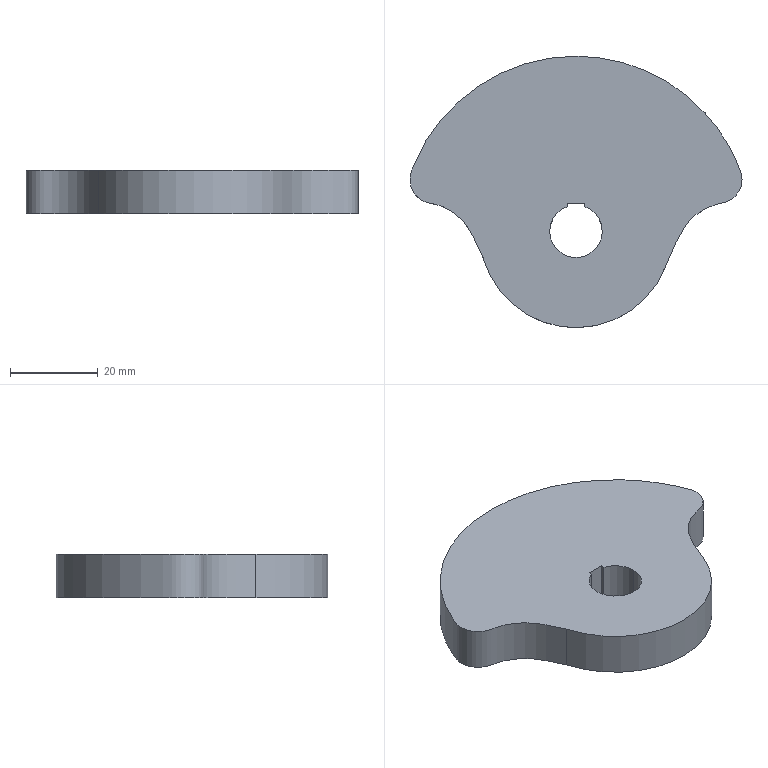Part | SolidWorks | features Extrusion 1, ICE 1 | 1 solid | 10 faces | box 75.848 x 62.021 x 10 mm | volume 29978 mm3 | plane 5 | cylinder 3 | spline 2 | commonest cylinder face diameters 12 x3
STEP:
#1=CARTESIAN_POINT('',(-6.,0.,0.));
#2=VERTEX_POINT('',#1);
#3=CARTESIAN_POINT('',(6.,0.,0.));
#4=VERTEX_POINT('',#3);
#5=CARTESIAN_POINT('',(0.,0.,0.));
#6=DIRECTION('',(0.,0.,1.));
#7=DIRECTION('',(-1.,0.,0.));
#8=AXIS2_PLACEMENT_3D('',#5,#6,#7);
#9=CIRCLE('',#8,6.);
#10=EDGE_CURVE('',#2,#4,#9,.T.);
#11=ORIENTED_EDGE('',*,*,#10,.F.);
#12=CARTESIAN_POINT('',(-6.,0.,10.));
#13=VERTEX_POINT('',#12);
#14=CARTESIAN_POINT('',(-6.,0.,-113.18));
#15=DIRECTION('',(0.,0.,1.));
#16=VECTOR('',#15,1000.);
#17=LINE('',#14,#16);
#18=EDGE_CURVE('',#2,#13,#17,.T.);
#19=ORIENTED_EDGE('',*,*,#18,.T.);
#20=CARTESIAN_POINT('',(6.,0.,10.));
#21=VERTEX_POINT('',#20);
#22=CARTESIAN_POINT('',(0.,0.,10.));
#23=DIRECTION('',(0.,0.,1.));
#24=DIRECTION('',(1.,0.,0.));
#25=AXIS2_PLACEMENT_3D('',#22,#23,#24);
#26=CIRCLE('',#25,6.);
#27=EDGE_CURVE('',#13,#21,#26,.T.);
#28=ORIENTED_EDGE('',*,*,#27,.T.);
#29=CARTESIAN_POINT('',(6.,0.,-113.18));
#30=DIRECTION('',(0.,0.,1.));
#31=VECTOR('',#30,1000.);
#32=LINE('',#29,#31);
#33=EDGE_CURVE('',#4,#21,#32,.T.);
#34=ORIENTED_EDGE('',*,*,#33,.F.);
#35=EDGE_LOOP('',(#11,#19,#28,#34));
#36=FACE_OUTER_BOUND('',#35,.T.);
#37=CARTESIAN_POINT('',(0.,0.,-113.18));
#38=DIRECTION('',(0.,0.,1.));
#39=DIRECTION('',(1.,0.,0.));
#40=AXIS2_PLACEMENT_3D('',#37,#38,#39);
#41=CYLINDRICAL_SURFACE('',#40,6.);
#42=ADVANCED_FACE('',(#36),#41,.F.);
#43=CARTESIAN_POINT('',(2.,5.657,0.));
#44=VERTEX_POINT('',#43);
#45=CARTESIAN_POINT('',(0.,0.,0.));
#46=DIRECTION('',(0.,0.,1.));
#47=DIRECTION('',(-1.,0.,0.));
#48=AXIS2_PLACEMENT_3D('',#45,#46,#47);
#49=CIRCLE('',#48,6.);
#50=EDGE_CURVE('',#4,#44,#49,.T.);
#51=ORIENTED_EDGE('',*,*,#50,.F.);
#52=ORIENTED_EDGE('',*,*,#33,.T.);
#53=CARTESIAN_POINT('',(2.,5.657,10.));
#54=VERTEX_POINT('',#53);
#55=CARTESIAN_POINT('',(0.,0.,10.));
#56=DIRECTION('',(0.,0.,1.));
#57=DIRECTION('',(1.,0.,0.));
#58=AXIS2_PLACEMENT_3D('',#55,#56,#57);
#59=CIRCLE('',#58,6.);
#60=EDGE_CURVE('',#21,#54,#59,.T.);
#61=ORIENTED_EDGE('',*,*,#60,.T.);
#62=CARTESIAN_POINT('',(2.,5.657,-113.18));
#63=DIRECTION('',(0.,0.,1.));
#64=VECTOR('',#63,1000.);
#65=LINE('',#62,#64);
#66=EDGE_CURVE('',#44,#54,#65,.T.);
#67=ORIENTED_EDGE('',*,*,#66,.F.);
#68=EDGE_LOOP('',(#51,#52,#61,#67));
#69=FACE_OUTER_BOUND('',#68,.T.);
#70=CARTESIAN_POINT('',(0.,0.,-113.18));
#71=DIRECTION('',(0.,0.,1.));
#72=DIRECTION('',(1.,0.,0.));
#73=AXIS2_PLACEMENT_3D('',#70,#71,#72);
#74=CYLINDRICAL_SURFACE('',#73,6.);
#75=ADVANCED_FACE('',(#69),#74,.F.);
#76=CARTESIAN_POINT('',(-21.423,-5.617,0.));
#77=VERTEX_POINT('',#76);
#78=CARTESIAN_POINT('',(29.487,27.043,0.));
#79=VERTEX_POINT('',#78);
#80=CARTESIAN_POINT('',(-21.423,-5.617,0.));
#81=CARTESIAN_POINT('',(-21.246,-6.047,0.));
#82=CARTESIAN_POINT('',(-20.905,-6.913,0.));
#83=CARTESIAN_POINT('',(-20.431,-8.228,0.));
#84=CARTESIAN_POINT('',(-20.056,-9.081,0.));
#85=CARTESIAN_POINT('',(-19.855,-9.501,0.));
#86=CARTESIAN_POINT('',(-10.656,-28.723,0.));
#87=CARTESIAN_POINT('',(10.654,-28.724,0.));
#88=CARTESIAN_POINT('',(19.854,-9.503,0.));
#89=CARTESIAN_POINT('',(20.055,-9.083,0.));
#90=CARTESIAN_POINT('',(20.43,-8.23,0.));
#91=CARTESIAN_POINT('',(20.904,-6.915,0.));
#92=CARTESIAN_POINT('',(21.246,-6.048,0.));
#93=CARTESIAN_POINT('',(21.422,-5.618,0.));
#94=CARTESIAN_POINT('',(21.978,-4.264,0.));
#95=CARTESIAN_POINT('',(22.591,-2.935,0.));
#96=CARTESIAN_POINT('',(23.261,-1.633,0.));
#97=CARTESIAN_POINT('',(23.355,-1.451,0.));
#98=CARTESIAN_POINT('',(23.545,-1.086,0.));
#99=CARTESIAN_POINT('',(23.838,-0.5418,0.));
#100=CARTESIAN_POINT('',(24.037,-0.1817,0.));
#101=CARTESIAN_POINT('',(24.138,-0.002216,0.));
#102=CARTESIAN_POINT('',(24.278,0.2481,0.));
#103=CARTESIAN_POINT('',(24.564,0.7463,0.));
#104=CARTESIAN_POINT('',(25.073,1.448,0.));
#105=CARTESIAN_POINT('',(25.433,1.896,0.));
#106=CARTESIAN_POINT('',(25.621,2.113,0.));
#107=CARTESIAN_POINT('',(27.42,4.203,0.));
#108=CARTESIAN_POINT('',(29.774,5.638,0.));
#109=CARTESIAN_POINT('',(32.456,6.278,0.));
#110=CARTESIAN_POINT('',(32.638,6.322,0.));
#111=CARTESIAN_POINT('',(33.005,6.401,0.));
#112=CARTESIAN_POINT('',(33.563,6.488,0.));
#113=CARTESIAN_POINT('',(33.927,6.581,0.));
#114=CARTESIAN_POINT('',(34.106,6.637,0.));
#115=CARTESIAN_POINT('',(36.786,7.474,0.));
#116=CARTESIAN_POINT('',(38.278,9.853,0.));
#117=CARTESIAN_POINT('',(37.865,12.631,0.));
#118=CARTESIAN_POINT('',(37.847,12.748,0.));
#119=CARTESIAN_POINT('',(37.805,12.98,0.));
#120=CARTESIAN_POINT('',(37.726,13.329,0.));
#121=CARTESIAN_POINT('',(37.646,13.552,0.));
#122=CARTESIAN_POINT('',(37.606,13.663,0.));
#123=CARTESIAN_POINT('',(37.565,13.775,0.));
#124=CARTESIAN_POINT('',(37.482,13.999,0.));
#125=CARTESIAN_POINT('',(37.356,14.333,0.));
#126=CARTESIAN_POINT('',(37.269,14.556,0.));
#127=CARTESIAN_POINT('',(37.226,14.667,0.));
#128=CARTESIAN_POINT('',(35.485,19.085,0.));
#129=CARTESIAN_POINT('',(32.926,23.294,0.));
#130=CARTESIAN_POINT('',(29.487,27.043,0.));
#131=(BOUNDED_CURVE()B_SPLINE_CURVE(3,(#80,#81,#82,#83,#84,#85,#86,#87,#88,#89,#90,#91,#92,#93,#94,#95,#96,#97,#98,#99,#100,#101,#102,#103,#104,#105,#106,#107,#108,#109,#110,#111,#112,#113,#114,#115,#116,#117,#118,#119,#120,#121,#122,#123,#124,#125,#126,#127,#128,#129,#130),.UNSPECIFIED.,.F.,.F.)B_SPLINE_CURVE_WITH_KNOTS((4,1,1,3,3,1,1,3,3,1,1,3,1,1,3,3,1,1,3,3,1,1,3,1,1,3,4),(0.,0.007845,0.01569,0.02353,0.2466,0.2545,0.2623,0.2702,0.2948,0.2983,0.3018,0.3052,0.3101,0.3149,0.3197,0.3647,0.3679,0.371,0.3742,0.4139,0.4159,0.4179,0.4199,0.4219,0.4239,0.4259,0.5),.UNSPECIFIED.)CURVE()GEOMETRIC_REPRESENTATION_ITEM()RATIONAL_B_SPLINE_CURVE((1.,1.,1.,1.,1.,1.,0.6211,0.6211,1.,1.,1.,1.,1.,1.,0.9994,0.9994,1.,1.,1.,1.,1.,1.,1.,1.,1.,1.,1.,0.9677,0.9677,1.,1.,1.,1.,1.,1.,0.8398,0.8398,1.,1.,1.,1.,1.,1.,1.,1.,1.,1.,1.,0.9252,0.8637,0.8154))REPRESENTATION_ITEM(''));
#132=EDGE_CURVE('',#77,#79,#131,.T.);
#133=ORIENTED_EDGE('',*,*,#132,.T.);
#134=CARTESIAN_POINT('',(29.487,27.043,10.));
#135=VERTEX_POINT('',#134);
#136=CARTESIAN_POINT('',(29.487,27.043,-113.18));
#137=DIRECTION('',(0.,0.,1.));
#138=VECTOR('',#137,1000.);
#139=LINE('',#136,#138);
#140=EDGE_CURVE('',#79,#135,#139,.T.);
#141=ORIENTED_EDGE('',*,*,#140,.T.);
#142=CARTESIAN_POINT('',(-21.423,-5.617,10.));
#143=VERTEX_POINT('',#142);
#144=CARTESIAN_POINT('',(-21.423,-5.617,10.));
#145=CARTESIAN_POINT('',(-21.246,-6.047,10.));
#146=CARTESIAN_POINT('',(-20.905,-6.913,10.));
#147=CARTESIAN_POINT('',(-20.431,-8.228,10.));
#148=CARTESIAN_POINT('',(-20.056,-9.081,10.));
#149=CARTESIAN_POINT('',(-19.855,-9.501,10.));
#150=CARTESIAN_POINT('',(-10.656,-28.723,10.));
#151=CARTESIAN_POINT('',(10.654,-28.724,10.));
#152=CARTESIAN_POINT('',(19.854,-9.503,10.));
#153=CARTESIAN_POINT('',(20.055,-9.083,10.));
#154=CARTESIAN_POINT('',(20.43,-8.23,10.));
#155=CARTESIAN_POINT('',(20.904,-6.915,10.));
#156=CARTESIAN_POINT('',(21.246,-6.048,10.));
#157=CARTESIAN_POINT('',(21.422,-5.618,10.));
#158=CARTESIAN_POINT('',(21.978,-4.264,10.));
#159=CARTESIAN_POINT('',(22.591,-2.935,10.));
#160=CARTESIAN_POINT('',(23.261,-1.633,10.));
#161=CARTESIAN_POINT('',(23.355,-1.451,10.));
#162=CARTESIAN_POINT('',(23.545,-1.086,10.));
#163=CARTESIAN_POINT('',(23.838,-0.5418,10.));
#164=CARTESIAN_POINT('',(24.037,-0.1817,10.));
#165=CARTESIAN_POINT('',(24.138,-0.002216,10.));
#166=CARTESIAN_POINT('',(24.278,0.2481,10.));
#167=CARTESIAN_POINT('',(24.564,0.7463,10.));
#168=CARTESIAN_POINT('',(25.073,1.448,10.));
#169=CARTESIAN_POINT('',(25.433,1.896,10.));
#170=CARTESIAN_POINT('',(25.621,2.113,10.));
#171=CARTESIAN_POINT('',(27.42,4.203,10.));
#172=CARTESIAN_POINT('',(29.774,5.638,10.));
#173=CARTESIAN_POINT('',(32.456,6.278,10.));
#174=CARTESIAN_POINT('',(32.638,6.322,10.));
#175=CARTESIAN_POINT('',(33.005,6.401,10.));
#176=CARTESIAN_POINT('',(33.563,6.488,10.));
#177=CARTESIAN_POINT('',(33.927,6.581,10.));
#178=CARTESIAN_POINT('',(34.106,6.637,10.));
#179=CARTESIAN_POINT('',(36.786,7.474,10.));
#180=CARTESIAN_POINT('',(38.278,9.853,10.));
#181=CARTESIAN_POINT('',(37.865,12.631,10.));
#182=CARTESIAN_POINT('',(37.847,12.748,10.));
#183=CARTESIAN_POINT('',(37.805,12.98,10.));
#184=CARTESIAN_POINT('',(37.726,13.329,10.));
#185=CARTESIAN_POINT('',(37.646,13.552,10.));
#186=CARTESIAN_POINT('',(37.606,13.663,10.));
#187=CARTESIAN_POINT('',(37.565,13.775,10.));
#188=CARTESIAN_POINT('',(37.482,13.999,10.));
#189=CARTESIAN_POINT('',(37.356,14.333,10.));
#190=CARTESIAN_POINT('',(37.269,14.556,10.));
#191=CARTESIAN_POINT('',(37.226,14.667,10.));
#192=CARTESIAN_POINT('',(35.485,19.085,10.));
#193=CARTESIAN_POINT('',(32.926,23.294,10.));
#194=CARTESIAN_POINT('',(29.487,27.043,10.));
#195=(BOUNDED_CURVE()B_SPLINE_CURVE(3,(#144,#145,#146,#147,#148,#149,#150,#151,#152,#153,#154,#155,#156,#157,#158,#159,#160,#161,#162,#163,#164,#165,#166,#167,#168,#169,#170,#171,#172,#173,#174,#175,#176,#177,#178,#179,#180,#181,#182,#183,#184,#185,#186,#187,#188,#189,#190,#191,#192,#193,#194),.UNSPECIFIED.,.F.,.F.)B_SPLINE_CURVE_WITH_KNOTS((4,1,1,3,3,1,1,3,3,1,1,3,1,1,3,3,1,1,3,3,1,1,3,1,1,3,4),(0.,0.007845,0.01569,0.02353,0.2466,0.2545,0.2623,0.2702,0.2948,0.2983,0.3018,0.3052,0.3101,0.3149,0.3197,0.3647,0.3679,0.371,0.3742,0.4139,0.4159,0.4179,0.4199,0.4219,0.4239,0.4259,0.5),.UNSPECIFIED.)CURVE()GEOMETRIC_REPRESENTATION_ITEM()RATIONAL_B_SPLINE_CURVE((1.,1.,1.,1.,1.,1.,0.6211,0.6211,1.,1.,1.,1.,1.,1.,0.9994,0.9994,1.,1.,1.,1.,1.,1.,1.,1.,1.,1.,1.,0.9677,0.9677,1.,1.,1.,1.,1.,1.,0.8398,0.8398,1.,1.,1.,1.,1.,1.,1.,1.,1.,1.,1.,0.9252,0.8637,0.8154))REPRESENTATION_ITEM(''));
#196=EDGE_CURVE('',#143,#135,#195,.T.);
#197=ORIENTED_EDGE('',*,*,#196,.F.);
#198=CARTESIAN_POINT('',(-21.423,-5.617,-113.18));
#199=DIRECTION('',(0.,0.,1.));
#200=VECTOR('',#199,1000.);
#201=LINE('',#198,#200);
#202=EDGE_CURVE('',#77,#143,#201,.T.);
#203=ORIENTED_EDGE('',*,*,#202,.F.);
#204=EDGE_LOOP('',(#133,#141,#197,#203));
#205=FACE_OUTER_BOUND('',#204,.T.);
#206=CARTESIAN_POINT('',(-21.423,-5.617,0.));
#207=CARTESIAN_POINT('',(-21.423,-5.617,10.));
#208=CARTESIAN_POINT('',(-21.246,-6.047,0.));
#209=CARTESIAN_POINT('',(-21.246,-6.047,10.));
#210=CARTESIAN_POINT('',(-20.905,-6.913,0.));
#211=CARTESIAN_POINT('',(-20.905,-6.913,10.));
#212=CARTESIAN_POINT('',(-20.431,-8.228,0.));
#213=CARTESIAN_POINT('',(-20.431,-8.228,10.));
#214=CARTESIAN_POINT('',(-20.056,-9.081,0.));
#215=CARTESIAN_POINT('',(-20.056,-9.081,10.));
#216=CARTESIAN_POINT('',(-19.855,-9.501,0.));
#217=CARTESIAN_POINT('',(-19.855,-9.501,10.));
#218=CARTESIAN_POINT('',(-10.656,-28.723,0.));
#219=CARTESIAN_POINT('',(-10.656,-28.723,10.));
#220=CARTESIAN_POINT('',(10.654,-28.724,0.));
#221=CARTESIAN_POINT('',(10.654,-28.724,10.));
#222=CARTESIAN_POINT('',(19.854,-9.503,0.));
#223=CARTESIAN_POINT('',(19.854,-9.503,10.));
#224=CARTESIAN_POINT('',(20.055,-9.083,0.));
#225=CARTESIAN_POINT('',(20.055,-9.083,10.));
#226=CARTESIAN_POINT('',(20.43,-8.23,0.));
#227=CARTESIAN_POINT('',(20.43,-8.23,10.));
#228=CARTESIAN_POINT('',(20.904,-6.915,0.));
#229=CARTESIAN_POINT('',(20.904,-6.915,10.));
#230=CARTESIAN_POINT('',(21.246,-6.048,0.));
#231=CARTESIAN_POINT('',(21.246,-6.048,10.));
#232=CARTESIAN_POINT('',(21.422,-5.618,0.));
#233=CARTESIAN_POINT('',(21.422,-5.618,10.));
#234=CARTESIAN_POINT('',(21.978,-4.264,0.));
#235=CARTESIAN_POINT('',(21.978,-4.264,10.));
#236=CARTESIAN_POINT('',(22.591,-2.935,0.));
#237=CARTESIAN_POINT('',(22.591,-2.935,10.));
#238=CARTESIAN_POINT('',(23.261,-1.633,0.));
#239=CARTESIAN_POINT('',(23.261,-1.633,10.));
#240=CARTESIAN_POINT('',(23.355,-1.451,0.));
#241=CARTESIAN_POINT('',(23.355,-1.451,10.));
#242=CARTESIAN_POINT('',(23.545,-1.086,0.));
#243=CARTESIAN_POINT('',(23.545,-1.086,10.));
#244=CARTESIAN_POINT('',(23.838,-0.5418,0.));
#245=CARTESIAN_POINT('',(23.838,-0.5418,10.));
#246=CARTESIAN_POINT('',(24.037,-0.1817,0.));
#247=CARTESIAN_POINT('',(24.037,-0.1817,10.));
#248=CARTESIAN_POINT('',(24.138,-0.002216,0.));
#249=CARTESIAN_POINT('',(24.138,-0.002216,10.));
#250=CARTESIAN_POINT('',(24.278,0.2481,0.));
#251=CARTESIAN_POINT('',(24.278,0.2481,10.));
#252=CARTESIAN_POINT('',(24.564,0.7463,0.));
#253=CARTESIAN_POINT('',(24.564,0.7463,10.));
#254=CARTESIAN_POINT('',(25.073,1.448,0.));
#255=CARTESIAN_POINT('',(25.073,1.448,10.));
#256=CARTESIAN_POINT('',(25.433,1.896,0.));
#257=CARTESIAN_POINT('',(25.433,1.896,10.));
#258=CARTESIAN_POINT('',(25.621,2.113,0.));
#259=CARTESIAN_POINT('',(25.621,2.113,10.));
#260=CARTESIAN_POINT('',(27.42,4.203,0.));
#261=CARTESIAN_POINT('',(27.42,4.203,10.));
#262=CARTESIAN_POINT('',(29.774,5.638,0.));
#263=CARTESIAN_POINT('',(29.774,5.638,10.));
#264=CARTESIAN_POINT('',(32.456,6.278,0.));
#265=CARTESIAN_POINT('',(32.456,6.278,10.));
#266=CARTESIAN_POINT('',(32.638,6.322,0.));
#267=CARTESIAN_POINT('',(32.638,6.322,10.));
#268=CARTESIAN_POINT('',(33.005,6.401,0.));
#269=CARTESIAN_POINT('',(33.005,6.401,10.));
#270=CARTESIAN_POINT('',(33.563,6.488,0.));
#271=CARTESIAN_POINT('',(33.563,6.488,10.));
#272=CARTESIAN_POINT('',(33.927,6.581,0.));
#273=CARTESIAN_POINT('',(33.927,6.581,10.));
#274=CARTESIAN_POINT('',(34.106,6.637,0.));
#275=CARTESIAN_POINT('',(34.106,6.637,10.));
#276=CARTESIAN_POINT('',(36.786,7.474,0.));
#277=CARTESIAN_POINT('',(36.786,7.474,10.));
#278=CARTESIAN_POINT('',(38.278,9.853,0.));
#279=CARTESIAN_POINT('',(38.278,9.853,10.));
#280=CARTESIAN_POINT('',(37.865,12.631,0.));
#281=CARTESIAN_POINT('',(37.865,12.631,10.));
#282=CARTESIAN_POINT('',(37.847,12.748,0.));
#283=CARTESIAN_POINT('',(37.847,12.748,10.));
#284=CARTESIAN_POINT('',(37.805,12.98,0.));
#285=CARTESIAN_POINT('',(37.805,12.98,10.));
#286=CARTESIAN_POINT('',(37.726,13.329,0.));
#287=CARTESIAN_POINT('',(37.726,13.329,10.));
#288=CARTESIAN_POINT('',(37.646,13.552,0.));
#289=CARTESIAN_POINT('',(37.646,13.552,10.));
#290=CARTESIAN_POINT('',(37.606,13.663,0.));
#291=CARTESIAN_POINT('',(37.606,13.663,10.));
#292=CARTESIAN_POINT('',(37.565,13.775,0.));
#293=CARTESIAN_POINT('',(37.565,13.775,10.));
#294=CARTESIAN_POINT('',(37.482,13.999,0.));
#295=CARTESIAN_POINT('',(37.482,13.999,10.));
#296=CARTESIAN_POINT('',(37.356,14.333,0.));
#297=CARTESIAN_POINT('',(37.356,14.333,10.));
#298=CARTESIAN_POINT('',(37.269,14.556,0.));
#299=CARTESIAN_POINT('',(37.269,14.556,10.));
#300=CARTESIAN_POINT('',(37.226,14.667,0.));
#301=CARTESIAN_POINT('',(37.226,14.667,10.));
#302=CARTESIAN_POINT('',(35.485,19.085,0.));
#303=CARTESIAN_POINT('',(35.485,19.085,10.));
#304=CARTESIAN_POINT('',(32.926,23.294,0.));
#305=CARTESIAN_POINT('',(32.926,23.294,10.));
#306=CARTESIAN_POINT('',(29.487,27.043,0.));
#307=CARTESIAN_POINT('',(29.487,27.043,10.));
#308=(BOUNDED_SURFACE()B_SPLINE_SURFACE(3,1,((#206,#207),(#208,#209),(#210,#211),(#212,#213),(#214,#215),(#216,#217),(#218,#219),(#220,#221),(#222,#223),(#224,#225),(#226,#227),(#228,#229),(#230,#231),(#232,#233),(#234,#235),(#236,#237),(#238,#239),(#240,#241),(#242,#243),(#244,#245),(#246,#247),(#248,#249),(#250,#251),(#252,#253),(#254,#255),(#256,#257),(#258,#259),(#260,#261),(#262,#263),(#264,#265),(#266,#267),(#268,#269),(#270,#271),(#272,#273),(#274,#275),(#276,#277),(#278,#279),(#280,#281),(#282,#283),(#284,#285),(#286,#287),(#288,#289),(#290,#291),(#292,#293),(#294,#295),(#296,#297),(#298,#299),(#300,#301),(#302,#303),(#304,#305),(#306,#307)),.UNSPECIFIED.,.F.,.F.,.T.)B_SPLINE_SURFACE_WITH_KNOTS((4,1,1,3,3,1,1,3,3,1,1,3,1,1,3,3,1,1,3,3,1,1,3,1,1,3,4),(2,2),(0.,0.007845,0.01569,0.02353,0.2466,0.2545,0.2623,0.2702,0.2948,0.2983,0.3018,0.3052,0.3101,0.3149,0.3197,0.3647,0.3679,0.371,0.3742,0.4139,0.4159,0.4179,0.4199,0.4219,0.4239,0.4259,0.5),(0.,1.),.UNSPECIFIED.)GEOMETRIC_REPRESENTATION_ITEM()RATIONAL_B_SPLINE_SURFACE(((1.,1.),(1.,1.),(1.,1.),(1.,1.),(1.,1.),(1.,1.),(0.6211,0.6211),(0.6211,0.6211),(1.,1.),(1.,1.),(1.,1.),(1.,1.),(1.,1.),(1.,1.),(0.9994,0.9994),(0.9994,0.9994),(1.,1.),(1.,1.),(1.,1.),(1.,1.),(1.,1.),(1.,1.),(1.,1.),(1.,1.),(1.,1.),(1.,1.),(1.,1.),(0.9677,0.9677),(0.9677,0.9677),(1.,1.),(1.,1.),(1.,1.),(1.,1.),(1.,1.),(1.,1.),(0.8398,0.8398),(0.8398,0.8398),(1.,1.),(1.,1.),(1.,1.),(1.,1.),(1.,1.),(1.,1.),(1.,1.),(1.,1.),(1.,1.),(1.,1.),(1.,1.),(0.9252,0.9252),(0.8637,0.8637),(0.8154,0.8154)))REPRESENTATION_ITEM('')SURFACE());
#309=ADVANCED_FACE('',(#205),#308,.T.);
#310=ORIENTED_EDGE('',*,*,#140,.F.);
#311=CARTESIAN_POINT('',(29.487,27.043,0.));
#312=CARTESIAN_POINT('',(6.127,52.515,0.));
#313=CARTESIAN_POINT('',(-25.753,43.789,0.));
#314=CARTESIAN_POINT('',(-37.226,14.665,0.));
#315=CARTESIAN_POINT('',(-37.27,14.555,0.));
#316=CARTESIAN_POINT('',(-37.356,14.332,0.));
#317=CARTESIAN_POINT('',(-37.483,13.998,0.));
#318=CARTESIAN_POINT('',(-37.565,13.774,0.));
#319=CARTESIAN_POINT('',(-37.606,13.662,0.));
#320=CARTESIAN_POINT('',(-37.646,13.551,0.));
#321=CARTESIAN_POINT('',(-37.726,13.329,0.));
#322=CARTESIAN_POINT('',(-37.805,12.981,0.));
#323=CARTESIAN_POINT('',(-37.847,12.749,0.));
#324=CARTESIAN_POINT('',(-37.864,12.632,0.));
#325=CARTESIAN_POINT('',(-38.279,9.854,0.));
#326=CARTESIAN_POINT('',(-36.787,7.474,0.));
#327=CARTESIAN_POINT('',(-34.106,6.637,0.));
#328=CARTESIAN_POINT('',(-33.927,6.581,0.));
#329=CARTESIAN_POINT('',(-33.563,6.488,0.));
#330=CARTESIAN_POINT('',(-33.005,6.401,0.));
#331=CARTESIAN_POINT('',(-32.638,6.322,0.));
#332=CARTESIAN_POINT('',(-32.456,6.278,0.));
#333=CARTESIAN_POINT('',(-29.773,5.637,0.));
#334=CARTESIAN_POINT('',(-27.418,4.202,0.));
#335=CARTESIAN_POINT('',(-25.619,2.112,0.));
#336=CARTESIAN_POINT('',(-25.432,1.895,0.));
#337=CARTESIAN_POINT('',(-25.073,1.447,0.));
#338=CARTESIAN_POINT('',(-24.564,0.7459,0.));
#339=CARTESIAN_POINT('',(-24.278,0.2481,0.));
#340=CARTESIAN_POINT('',(-24.138,-0.001969,0.));
#341=CARTESIAN_POINT('',(-24.037,-0.1813,0.));
#342=CARTESIAN_POINT('',(-23.838,-0.5411,0.));
#343=CARTESIAN_POINT('',(-23.546,-1.085,0.));
#344=CARTESIAN_POINT('',(-23.355,-1.449,0.));
#345=CARTESIAN_POINT('',(-23.261,-1.632,0.));
#346=CARTESIAN_POINT('',(-22.592,-2.933,0.));
#347=CARTESIAN_POINT('',(-21.978,-4.262,0.));
#348=CARTESIAN_POINT('',(-21.423,-5.617,0.));
#349=(BOUNDED_CURVE()B_SPLINE_CURVE(3,(#311,#312,#313,#314,#315,#316,#317,#318,#319,#320,#321,#322,#323,#324,#325,#326,#327,#328,#329,#330,#331,#332,#333,#334,#335,#336,#337,#338,#339,#340,#341,#342,#343,#344,#345,#346,#347,#348),.UNSPECIFIED.,.F.,.T.)B_SPLINE_CURVE_WITH_KNOTS((4,3,1,1,3,1,1,3,3,1,1,3,3,1,1,3,1,1,3,4),(0.5,0.8442,0.8462,0.8482,0.8503,0.8522,0.8542,0.8562,0.896,0.8991,0.9023,0.9055,0.9504,0.9553,0.9601,0.9649,0.9684,0.9719,0.9753,1.),.UNSPECIFIED.)CURVE()GEOMETRIC_REPRESENTATION_ITEM()RATIONAL_B_SPLINE_CURVE((0.8154,0.5909,0.6525,1.,1.,1.,1.,1.,1.,1.,1.,1.,1.,1.,0.8397,0.8397,1.,1.,1.,1.,1.,1.,0.9676,0.9676,1.,1.,1.,1.,1.,1.,1.,1.,1.,1.,1.,0.9994,0.9994,1.))REPRESENTATION_ITEM(''));
#350=EDGE_CURVE('',#79,#77,#349,.T.);
#351=ORIENTED_EDGE('',*,*,#350,.T.);
#352=ORIENTED_EDGE('',*,*,#202,.T.);
#353=CARTESIAN_POINT('',(29.487,27.043,10.));
#354=CARTESIAN_POINT('',(6.127,52.515,10.));
#355=CARTESIAN_POINT('',(-25.753,43.789,10.));
#356=CARTESIAN_POINT('',(-37.226,14.665,10.));
#357=CARTESIAN_POINT('',(-37.27,14.555,10.));
#358=CARTESIAN_POINT('',(-37.356,14.332,10.));
#359=CARTESIAN_POINT('',(-37.483,13.998,10.));
#360=CARTESIAN_POINT('',(-37.565,13.774,10.));
#361=CARTESIAN_POINT('',(-37.606,13.662,10.));
#362=CARTESIAN_POINT('',(-37.646,13.551,10.));
#363=CARTESIAN_POINT('',(-37.726,13.329,10.));
#364=CARTESIAN_POINT('',(-37.805,12.981,10.));
#365=CARTESIAN_POINT('',(-37.847,12.749,10.));
#366=CARTESIAN_POINT('',(-37.864,12.632,10.));
#367=CARTESIAN_POINT('',(-38.279,9.854,10.));
#368=CARTESIAN_POINT('',(-36.787,7.474,10.));
#369=CARTESIAN_POINT('',(-34.106,6.637,10.));
#370=CARTESIAN_POINT('',(-33.927,6.581,10.));
#371=CARTESIAN_POINT('',(-33.563,6.488,10.));
#372=CARTESIAN_POINT('',(-33.005,6.401,10.));
#373=CARTESIAN_POINT('',(-32.638,6.322,10.));
#374=CARTESIAN_POINT('',(-32.456,6.278,10.));
#375=CARTESIAN_POINT('',(-29.773,5.637,10.));
#376=CARTESIAN_POINT('',(-27.418,4.202,10.));
#377=CARTESIAN_POINT('',(-25.619,2.112,10.));
#378=CARTESIAN_POINT('',(-25.432,1.895,10.));
#379=CARTESIAN_POINT('',(-25.073,1.447,10.));
#380=CARTESIAN_POINT('',(-24.564,0.7459,10.));
#381=CARTESIAN_POINT('',(-24.278,0.2481,10.));
#382=CARTESIAN_POINT('',(-24.138,-0.001969,10.));
#383=CARTESIAN_POINT('',(-24.037,-0.1813,10.));
#384=CARTESIAN_POINT('',(-23.838,-0.5411,10.));
#385=CARTESIAN_POINT('',(-23.546,-1.085,10.));
#386=CARTESIAN_POINT('',(-23.355,-1.449,10.));
#387=CARTESIAN_POINT('',(-23.261,-1.632,10.));
#388=CARTESIAN_POINT('',(-22.592,-2.933,10.));
#389=CARTESIAN_POINT('',(-21.978,-4.262,10.));
#390=CARTESIAN_POINT('',(-21.423,-5.617,10.));
#391=(BOUNDED_CURVE()B_SPLINE_CURVE(3,(#353,#354,#355,#356,#357,#358,#359,#360,#361,#362,#363,#364,#365,#366,#367,#368,#369,#370,#371,#372,#373,#374,#375,#376,#377,#378,#379,#380,#381,#382,#383,#384,#385,#386,#387,#388,#389,#390),.UNSPECIFIED.,.F.,.F.)B_SPLINE_CURVE_WITH_KNOTS((4,3,1,1,3,1,1,3,3,1,1,3,3,1,1,3,1,1,3,4),(0.5,0.8442,0.8462,0.8482,0.8503,0.8522,0.8542,0.8562,0.896,0.8991,0.9023,0.9055,0.9504,0.9553,0.9601,0.9649,0.9684,0.9719,0.9753,1.),.UNSPECIFIED.)CURVE()GEOMETRIC_REPRESENTATION_ITEM()RATIONAL_B_SPLINE_CURVE((0.8154,0.5909,0.6525,1.,1.,1.,1.,1.,1.,1.,1.,1.,1.,1.,0.8397,0.8397,1.,1.,1.,1.,1.,1.,0.9676,0.9676,1.,1.,1.,1.,1.,1.,1.,1.,1.,1.,1.,0.9994,0.9994,1.))REPRESENTATION_ITEM(''));
#392=EDGE_CURVE('',#135,#143,#391,.T.);
#393=ORIENTED_EDGE('',*,*,#392,.F.);
#394=EDGE_LOOP('',(#310,#351,#352,#393));
#395=FACE_OUTER_BOUND('',#394,.T.);
#396=CARTESIAN_POINT('',(29.487,27.043,0.));
#397=CARTESIAN_POINT('',(29.487,27.043,10.));
#398=CARTESIAN_POINT('',(6.127,52.515,0.));
#399=CARTESIAN_POINT('',(6.127,52.515,10.));
#400=CARTESIAN_POINT('',(-25.753,43.789,0.));
#401=CARTESIAN_POINT('',(-25.753,43.789,10.));
#402=CARTESIAN_POINT('',(-37.226,14.665,0.));
#403=CARTESIAN_POINT('',(-37.226,14.665,10.));
#404=CARTESIAN_POINT('',(-37.27,14.555,0.));
#405=CARTESIAN_POINT('',(-37.27,14.555,10.));
#406=CARTESIAN_POINT('',(-37.356,14.332,0.));
#407=CARTESIAN_POINT('',(-37.356,14.332,10.));
#408=CARTESIAN_POINT('',(-37.483,13.998,0.));
#409=CARTESIAN_POINT('',(-37.483,13.998,10.));
#410=CARTESIAN_POINT('',(-37.565,13.774,0.));
#411=CARTESIAN_POINT('',(-37.565,13.774,10.));
#412=CARTESIAN_POINT('',(-37.606,13.662,0.));
#413=CARTESIAN_POINT('',(-37.606,13.662,10.));
#414=CARTESIAN_POINT('',(-37.646,13.551,0.));
#415=CARTESIAN_POINT('',(-37.646,13.551,10.));
#416=CARTESIAN_POINT('',(-37.726,13.329,0.));
#417=CARTESIAN_POINT('',(-37.726,13.329,10.));
#418=CARTESIAN_POINT('',(-37.805,12.981,0.));
#419=CARTESIAN_POINT('',(-37.805,12.981,10.));
#420=CARTESIAN_POINT('',(-37.847,12.749,0.));
#421=CARTESIAN_POINT('',(-37.847,12.749,10.));
#422=CARTESIAN_POINT('',(-37.864,12.632,0.));
#423=CARTESIAN_POINT('',(-37.864,12.632,10.));
#424=CARTESIAN_POINT('',(-38.279,9.854,0.));
#425=CARTESIAN_POINT('',(-38.279,9.854,10.));
#426=CARTESIAN_POINT('',(-36.787,7.474,0.));
#427=CARTESIAN_POINT('',(-36.787,7.474,10.));
#428=CARTESIAN_POINT('',(-34.106,6.637,0.));
#429=CARTESIAN_POINT('',(-34.106,6.637,10.));
#430=CARTESIAN_POINT('',(-33.927,6.581,0.));
#431=CARTESIAN_POINT('',(-33.927,6.581,10.));
#432=CARTESIAN_POINT('',(-33.563,6.488,0.));
#433=CARTESIAN_POINT('',(-33.563,6.488,10.));
#434=CARTESIAN_POINT('',(-33.005,6.401,0.));
#435=CARTESIAN_POINT('',(-33.005,6.401,10.));
#436=CARTESIAN_POINT('',(-32.638,6.322,0.));
#437=CARTESIAN_POINT('',(-32.638,6.322,10.));
#438=CARTESIAN_POINT('',(-32.456,6.278,0.));
#439=CARTESIAN_POINT('',(-32.456,6.278,10.));
#440=CARTESIAN_POINT('',(-29.773,5.637,0.));
#441=CARTESIAN_POINT('',(-29.773,5.637,10.));
#442=CARTESIAN_POINT('',(-27.418,4.202,0.));
#443=CARTESIAN_POINT('',(-27.418,4.202,10.));
#444=CARTESIAN_POINT('',(-25.619,2.112,0.));
#445=CARTESIAN_POINT('',(-25.619,2.112,10.));
#446=CARTESIAN_POINT('',(-25.432,1.895,0.));
#447=CARTESIAN_POINT('',(-25.432,1.895,10.));
#448=CARTESIAN_POINT('',(-25.073,1.447,0.));
#449=CARTESIAN_POINT('',(-25.073,1.447,10.));
#450=CARTESIAN_POINT('',(-24.564,0.7459,0.));
#451=CARTESIAN_POINT('',(-24.564,0.7459,10.));
#452=CARTESIAN_POINT('',(-24.278,0.2481,0.));
#453=CARTESIAN_POINT('',(-24.278,0.2481,10.));
#454=CARTESIAN_POINT('',(-24.138,-0.001969,0.));
#455=CARTESIAN_POINT('',(-24.138,-0.001969,10.));
#456=CARTESIAN_POINT('',(-24.037,-0.1813,0.));
#457=CARTESIAN_POINT('',(-24.037,-0.1813,10.));
#458=CARTESIAN_POINT('',(-23.838,-0.5411,0.));
#459=CARTESIAN_POINT('',(-23.838,-0.5411,10.));
#460=CARTESIAN_POINT('',(-23.546,-1.085,0.));
#461=CARTESIAN_POINT('',(-23.546,-1.085,10.));
#462=CARTESIAN_POINT('',(-23.355,-1.449,0.));
#463=CARTESIAN_POINT('',(-23.355,-1.449,10.));
#464=CARTESIAN_POINT('',(-23.261,-1.632,0.));
#465=CARTESIAN_POINT('',(-23.261,-1.632,10.));
#466=CARTESIAN_POINT('',(-22.592,-2.933,0.));
#467=CARTESIAN_POINT('',(-22.592,-2.933,10.));
#468=CARTESIAN_POINT('',(-21.978,-4.262,0.));
#469=CARTESIAN_POINT('',(-21.978,-4.262,10.));
#470=CARTESIAN_POINT('',(-21.423,-5.617,0.));
#471=CARTESIAN_POINT('',(-21.423,-5.617,10.));
#472=(BOUNDED_SURFACE()B_SPLINE_SURFACE(3,1,((#396,#397),(#398,#399),(#400,#401),(#402,#403),(#404,#405),(#406,#407),(#408,#409),(#410,#411),(#412,#413),(#414,#415),(#416,#417),(#418,#419),(#420,#421),(#422,#423),(#424,#425),(#426,#427),(#428,#429),(#430,#431),(#432,#433),(#434,#435),(#436,#437),(#438,#439),(#440,#441),(#442,#443),(#444,#445),(#446,#447),(#448,#449),(#450,#451),(#452,#453),(#454,#455),(#456,#457),(#458,#459),(#460,#461),(#462,#463),(#464,#465),(#466,#467),(#468,#469),(#470,#471)),.UNSPECIFIED.,.F.,.F.,.T.)B_SPLINE_SURFACE_WITH_KNOTS((4,3,1,1,3,1,1,3,3,1,1,3,3,1,1,3,1,1,3,4),(2,2),(0.5,0.8442,0.8462,0.8482,0.8503,0.8522,0.8542,0.8562,0.896,0.8991,0.9023,0.9055,0.9504,0.9553,0.9601,0.9649,0.9684,0.9719,0.9753,1.),(0.,1.),.UNSPECIFIED.)GEOMETRIC_REPRESENTATION_ITEM()RATIONAL_B_SPLINE_SURFACE(((0.8154,0.8154),(0.5909,0.5909),(0.6525,0.6525),(1.,1.),(1.,1.),(1.,1.),(1.,1.),(1.,1.),(1.,1.),(1.,1.),(1.,1.),(1.,1.),(1.,1.),(1.,1.),(0.8397,0.8397),(0.8397,0.8397),(1.,1.),(1.,1.),(1.,1.),(1.,1.),(1.,1.),(1.,1.),(0.9676,0.9676),(0.9676,0.9676),(1.,1.),(1.,1.),(1.,1.),(1.,1.),(1.,1.),(1.,1.),(1.,1.),(1.,1.),(1.,1.),(1.,1.),(1.,1.),(0.9994,0.9994),(0.9994,0.9994),(1.,1.)))REPRESENTATION_ITEM('')SURFACE());
#473=ADVANCED_FACE('',(#395),#472,.T.);
#474=CARTESIAN_POINT('',(2.,6.472,0.));
#475=VERTEX_POINT('',#474);
#476=CARTESIAN_POINT('',(-2.,6.472,0.));
#477=VERTEX_POINT('',#476);
#478=CARTESIAN_POINT('',(2.,6.472,0.));
#479=DIRECTION('',(-1.,0.,0.));
#480=VECTOR('',#479,1000.);
#481=LINE('',#478,#480);
#482=EDGE_CURVE('',#475,#477,#481,.T.);
#483=ORIENTED_EDGE('',*,*,#482,.F.);
#484=CARTESIAN_POINT('',(2.,6.472,10.));
#485=VERTEX_POINT('',#484);
#486=CARTESIAN_POINT('',(2.,6.472,-113.18));
#487=DIRECTION('',(0.,0.,1.));
#488=VECTOR('',#487,1000.);
#489=LINE('',#486,#488);
#490=EDGE_CURVE('',#475,#485,#489,.T.);
#491=ORIENTED_EDGE('',*,*,#490,.T.);
#492=CARTESIAN_POINT('',(-2.,6.472,10.));
#493=VERTEX_POINT('',#492);
#494=CARTESIAN_POINT('',(2.,6.472,10.));
#495=DIRECTION('',(-1.,0.,0.));
#496=VECTOR('',#495,1000.);
#497=LINE('',#494,#496);
#498=EDGE_CURVE('',#485,#493,#497,.T.);
#499=ORIENTED_EDGE('',*,*,#498,.T.);
#500=CARTESIAN_POINT('',(-2.,6.472,-113.18));
#501=DIRECTION('',(0.,0.,1.));
#502=VECTOR('',#501,1000.);
#503=LINE('',#500,#502);
#504=EDGE_CURVE('',#477,#493,#503,.T.);
#505=ORIENTED_EDGE('',*,*,#504,.F.);
#506=EDGE_LOOP('',(#483,#491,#499,#505));
#507=FACE_OUTER_BOUND('',#506,.T.);
#508=CARTESIAN_POINT('',(2.,6.472,-113.18));
#509=DIRECTION('',(0.,1.,0.));
#510=DIRECTION('',(-1.,0.,0.));
#511=AXIS2_PLACEMENT_3D('',#508,#509,#510);
#512=PLANE('',#511);
#513=ADVANCED_FACE('',(#507),#512,.F.);
#514=CARTESIAN_POINT('',(2.,5.657,0.));
#515=DIRECTION('',(0.,1.,0.));
#516=VECTOR('',#515,1000.);
#517=LINE('',#514,#516);
#518=EDGE_CURVE('',#44,#475,#517,.T.);
#519=ORIENTED_EDGE('',*,*,#518,.F.);
#520=ORIENTED_EDGE('',*,*,#66,.T.);
#521=CARTESIAN_POINT('',(2.,5.657,10.));
#522=DIRECTION('',(0.,1.,0.));
#523=VECTOR('',#522,1000.);
#524=LINE('',#521,#523);
#525=EDGE_CURVE('',#54,#485,#524,.T.);
#526=ORIENTED_EDGE('',*,*,#525,.T.);
#527=ORIENTED_EDGE('',*,*,#490,.F.);
#528=EDGE_LOOP('',(#519,#520,#526,#527));
#529=FACE_OUTER_BOUND('',#528,.T.);
#530=CARTESIAN_POINT('',(2.,5.657,-113.18));
#531=DIRECTION('',(1.,0.,0.));
#532=DIRECTION('',(0.,0.,-1.));
#533=AXIS2_PLACEMENT_3D('',#530,#531,#532);
#534=PLANE('',#533);
#535=ADVANCED_FACE('',(#529),#534,.F.);
#536=ORIENTED_EDGE('',*,*,#18,.F.);
#537=CARTESIAN_POINT('',(-2.,5.657,0.));
#538=VERTEX_POINT('',#537);
#539=CARTESIAN_POINT('',(0.,0.,0.));
#540=DIRECTION('',(0.,0.,1.));
#541=DIRECTION('',(-1.,0.,0.));
#542=AXIS2_PLACEMENT_3D('',#539,#540,#541);
#543=CIRCLE('',#542,6.);
#544=EDGE_CURVE('',#538,#2,#543,.T.);
#545=ORIENTED_EDGE('',*,*,#544,.F.);
#546=CARTESIAN_POINT('',(-2.,5.657,10.));
#547=VERTEX_POINT('',#546);
#548=CARTESIAN_POINT('',(-2.,5.657,-113.18));
#549=DIRECTION('',(0.,0.,1.));
#550=VECTOR('',#549,1000.);
#551=LINE('',#548,#550);
#552=EDGE_CURVE('',#538,#547,#551,.T.);
#553=ORIENTED_EDGE('',*,*,#552,.T.);
#554=CARTESIAN_POINT('',(0.,0.,10.));
#555=DIRECTION('',(0.,0.,1.));
#556=DIRECTION('',(1.,0.,0.));
#557=AXIS2_PLACEMENT_3D('',#554,#555,#556);
#558=CIRCLE('',#557,6.);
#559=EDGE_CURVE('',#547,#13,#558,.T.);
#560=ORIENTED_EDGE('',*,*,#559,.T.);
#561=EDGE_LOOP('',(#536,#545,#553,#560));
#562=FACE_OUTER_BOUND('',#561,.T.);
#563=CARTESIAN_POINT('',(0.,0.,-113.18));
#564=DIRECTION('',(0.,0.,1.));
#565=DIRECTION('',(1.,0.,0.));
#566=AXIS2_PLACEMENT_3D('',#563,#564,#565);
#567=CYLINDRICAL_SURFACE('',#566,6.);
#568=ADVANCED_FACE('',(#562),#567,.F.);
#569=CARTESIAN_POINT('',(-2.,6.472,0.));
#570=DIRECTION('',(0.,-1.,0.));
#571=VECTOR('',#570,1000.);
#572=LINE('',#569,#571);
#573=EDGE_CURVE('',#477,#538,#572,.T.);
#574=ORIENTED_EDGE('',*,*,#573,.F.);
#575=ORIENTED_EDGE('',*,*,#504,.T.);
#576=CARTESIAN_POINT('',(-2.,6.472,10.));
#577=DIRECTION('',(0.,-1.,0.));
#578=VECTOR('',#577,1000.);
#579=LINE('',#576,#578);
#580=EDGE_CURVE('',#493,#547,#579,.T.);
#581=ORIENTED_EDGE('',*,*,#580,.T.);
#582=ORIENTED_EDGE('',*,*,#552,.F.);
#583=EDGE_LOOP('',(#574,#575,#581,#582));
#584=FACE_OUTER_BOUND('',#583,.T.);
#585=CARTESIAN_POINT('',(-2.,6.472,-113.18));
#586=DIRECTION('',(-1.,0.,0.));
#587=DIRECTION('',(0.,-1.,0.));
#588=AXIS2_PLACEMENT_3D('',#585,#586,#587);
#589=PLANE('',#588);
#590=ADVANCED_FACE('',(#584),#589,.F.);
#591=ORIENTED_EDGE('',*,*,#580,.F.);
#592=ORIENTED_EDGE('',*,*,#498,.F.);
#593=ORIENTED_EDGE('',*,*,#525,.F.);
#594=ORIENTED_EDGE('',*,*,#60,.F.);
#595=ORIENTED_EDGE('',*,*,#27,.F.);
#596=ORIENTED_EDGE('',*,*,#559,.F.);
#597=EDGE_LOOP('',(#591,#592,#593,#594,#595,#596));
#598=FACE_BOUND('',#597,.T.);
#599=ORIENTED_EDGE('',*,*,#196,.T.);
#600=ORIENTED_EDGE('',*,*,#392,.T.);
#601=EDGE_LOOP('',(#599,#600));
#602=FACE_OUTER_BOUND('',#601,.T.);
#603=CARTESIAN_POINT('',(29.487,27.043,10.));
#604=DIRECTION('',(0.,0.,-1.));
#605=DIRECTION('',(-1.,0.,0.));
#606=AXIS2_PLACEMENT_3D('',#603,#604,#605);
#607=PLANE('',#606);
#608=ADVANCED_FACE('',(#598,#602),#607,.F.);
#609=ORIENTED_EDGE('',*,*,#132,.F.);
#610=ORIENTED_EDGE('',*,*,#350,.F.);
#611=EDGE_LOOP('',(#609,#610));
#612=FACE_OUTER_BOUND('',#611,.T.);
#613=ORIENTED_EDGE('',*,*,#518,.T.);
#614=ORIENTED_EDGE('',*,*,#482,.T.);
#615=ORIENTED_EDGE('',*,*,#573,.T.);
#616=ORIENTED_EDGE('',*,*,#544,.T.);
#617=ORIENTED_EDGE('',*,*,#10,.T.);
#618=ORIENTED_EDGE('',*,*,#50,.T.);
#619=EDGE_LOOP('',(#613,#614,#615,#616,#617,#618));
#620=FACE_BOUND('',#619,.T.);
#621=CARTESIAN_POINT('',(-34.303,-12.485,0.));
#622=DIRECTION('',(0.,0.,-1.));
#623=DIRECTION('',(-1.,0.,0.));
#624=AXIS2_PLACEMENT_3D('',#621,#622,#623);
#625=PLANE('',#624);
#626=ADVANCED_FACE('',(#612,#620),#625,.T.);
#627=CLOSED_SHELL('',(#42,#75,#309,#473,#513,#535,#568,#590,#608,#626));
#628=MANIFOLD_SOLID_BREP('',#627);
#629=CARTESIAN_POINT('',(0.,0.,0.));
#630=DIRECTION('',(0.,0.,1.));
#631=DIRECTION('',(1.,0.,0.));
#632=AXIS2_PLACEMENT_3D('',#629,#630,#631);
#633=(LENGTH_UNIT()NAMED_UNIT(*)SI_UNIT(.MILLI.,.METRE.));
#634=UNCERTAINTY_MEASURE_WITH_UNIT(LENGTH_MEASURE(0.00001),#633,'','');
#635=(NAMED_UNIT(*)PLANE_ANGLE_UNIT()SI_UNIT($,.RADIAN.));
#636=(NAMED_UNIT(*)SI_UNIT($,.STERADIAN.)SOLID_ANGLE_UNIT());
#637=(GEOMETRIC_REPRESENTATION_CONTEXT(3)GLOBAL_UNCERTAINTY_ASSIGNED_CONTEXT((#634))GLOBAL_UNIT_ASSIGNED_CONTEXT((#633,#635,#636))REPRESENTATION_CONTEXT('',''));
#638=ADVANCED_BREP_SHAPE_REPRESENTATION('',(#628,#632),#637);